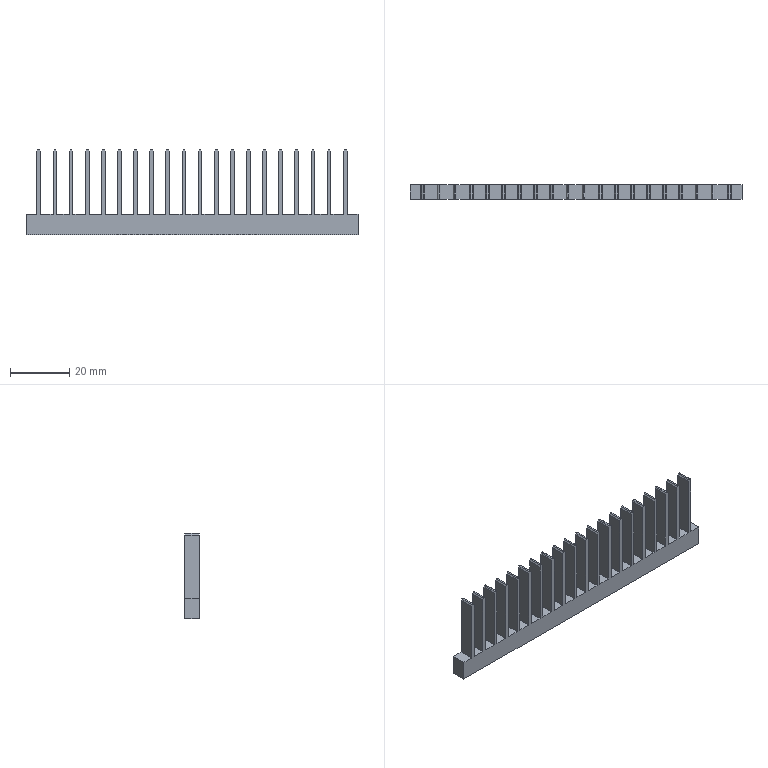Part | STEP file | 1 solid | 126 faces | box 112 x 4.97 x 28.8 mm | volume 6489 mm3 | plane 106 | cylinder 20 | commonest cylinder face diameters 0.68 x20